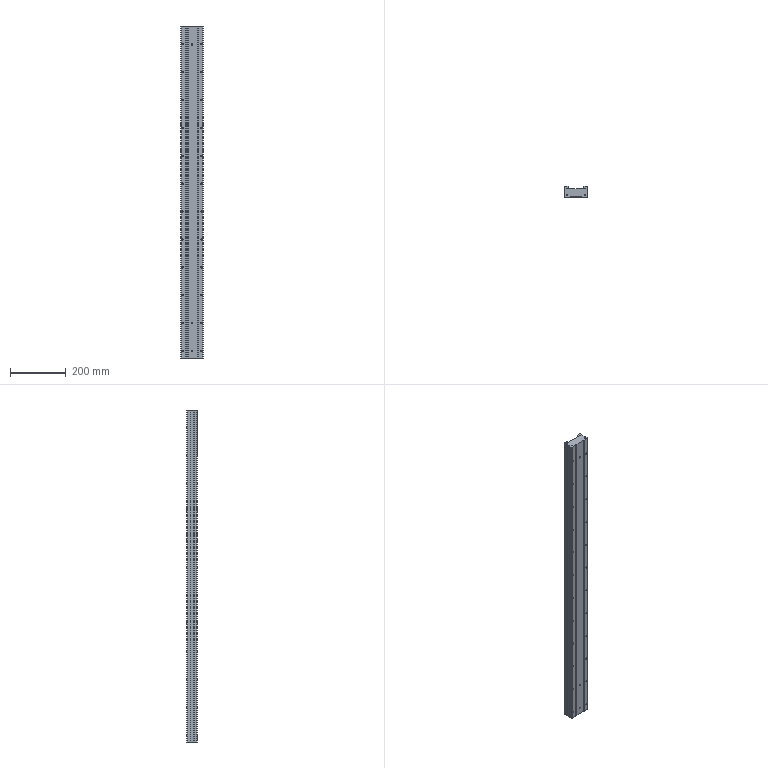Part | NX | features BREP 1 | 1 solid | 230 faces | box 82 x 38 x 1190 mm | volume 3089762 mm3 | cylinder 126 | cone 64 | plane 40 | commonest cylinder face diameters 5 x55 5.4 x48 3.3 x16 0.6 x6 3 x1